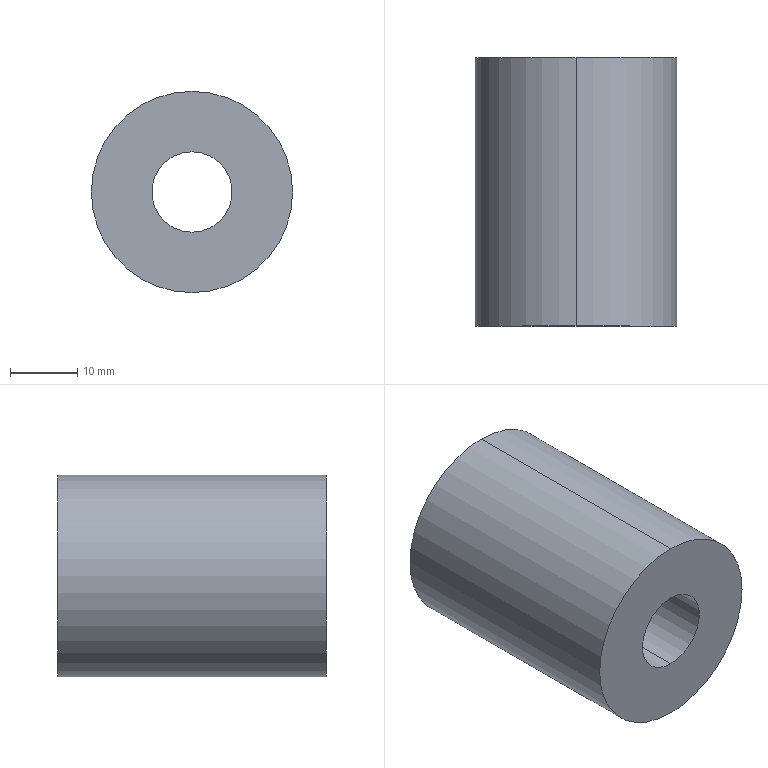Part | SolidWorks | features BaseBody 1 | 1 solid | 6 faces | box 30 x 40 x 30 mm | volume 23750 mm3 | cylinder 4 | plane 2 | commonest cylinder face diameters 12 x2 30 x2
STEP:
#1=CARTESIAN_POINT('',(0.,40.,-15.));
#2=VERTEX_POINT('',#1);
#3=CARTESIAN_POINT('',(0.,40.,15.));
#4=VERTEX_POINT('',#3);
#5=CARTESIAN_POINT('',(0.,40.,0.));
#6=DIRECTION('',(0.,-1.,0.));
#7=DIRECTION('',(0.,0.,-1.));
#8=AXIS2_PLACEMENT_3D('',#5,#6,#7);
#9=CIRCLE('',#8,15.);
#10=EDGE_CURVE('',#2,#4,#9,.T.);
#11=ORIENTED_EDGE('',*,*,#10,.T.);
#12=CARTESIAN_POINT('',(0.,0.,15.));
#13=VERTEX_POINT('',#12);
#14=CARTESIAN_POINT('',(0.,40.,15.));
#15=DIRECTION('',(0.,-1.,0.));
#16=VECTOR('',#15,1000.);
#17=LINE('',#14,#16);
#18=EDGE_CURVE('',#4,#13,#17,.T.);
#19=ORIENTED_EDGE('',*,*,#18,.T.);
#20=CARTESIAN_POINT('',(0.,0.,-15.));
#21=VERTEX_POINT('',#20);
#22=CARTESIAN_POINT('',(0.,0.,0.));
#23=DIRECTION('',(0.,1.,0.));
#24=DIRECTION('',(0.,0.,-1.));
#25=AXIS2_PLACEMENT_3D('',#22,#23,#24);
#26=CIRCLE('',#25,15.);
#27=EDGE_CURVE('',#13,#21,#26,.T.);
#28=ORIENTED_EDGE('',*,*,#27,.T.);
#29=CARTESIAN_POINT('',(0.,40.,-15.));
#30=DIRECTION('',(0.,-1.,0.));
#31=VECTOR('',#30,1000.);
#32=LINE('',#29,#31);
#33=EDGE_CURVE('',#2,#21,#32,.T.);
#34=ORIENTED_EDGE('',*,*,#33,.F.);
#35=EDGE_LOOP('',(#11,#19,#28,#34));
#36=FACE_OUTER_BOUND('',#35,.T.);
#37=CARTESIAN_POINT('',(0.,40.,0.));
#38=DIRECTION('',(0.,-1.,0.));
#39=DIRECTION('',(0.,0.,-1.));
#40=AXIS2_PLACEMENT_3D('',#37,#38,#39);
#41=CYLINDRICAL_SURFACE('',#40,15.);
#42=ADVANCED_FACE('',(#36),#41,.T.);
#43=CARTESIAN_POINT('',(0.,40.,6.));
#44=VERTEX_POINT('',#43);
#45=CARTESIAN_POINT('',(0.,40.,-6.));
#46=VERTEX_POINT('',#45);
#47=CARTESIAN_POINT('',(0.,40.,0.));
#48=DIRECTION('',(0.,-1.,0.));
#49=DIRECTION('',(0.,0.,-1.));
#50=AXIS2_PLACEMENT_3D('',#47,#48,#49);
#51=CIRCLE('',#50,6.);
#52=EDGE_CURVE('',#44,#46,#51,.T.);
#53=ORIENTED_EDGE('',*,*,#52,.F.);
#54=CARTESIAN_POINT('',(0.,0.,6.));
#55=VERTEX_POINT('',#54);
#56=CARTESIAN_POINT('',(0.,40.,6.));
#57=DIRECTION('',(0.,-1.,0.));
#58=VECTOR('',#57,1000.);
#59=LINE('',#56,#58);
#60=EDGE_CURVE('',#44,#55,#59,.T.);
#61=ORIENTED_EDGE('',*,*,#60,.T.);
#62=CARTESIAN_POINT('',(0.,0.,-6.));
#63=VERTEX_POINT('',#62);
#64=CARTESIAN_POINT('',(0.,0.,0.));
#65=DIRECTION('',(0.,-1.,0.));
#66=DIRECTION('',(0.,0.,-1.));
#67=AXIS2_PLACEMENT_3D('',#64,#65,#66);
#68=CIRCLE('',#67,6.);
#69=EDGE_CURVE('',#55,#63,#68,.T.);
#70=ORIENTED_EDGE('',*,*,#69,.T.);
#71=CARTESIAN_POINT('',(0.,40.,-6.));
#72=DIRECTION('',(0.,-1.,0.));
#73=VECTOR('',#72,1000.);
#74=LINE('',#71,#73);
#75=EDGE_CURVE('',#46,#63,#74,.T.);
#76=ORIENTED_EDGE('',*,*,#75,.F.);
#77=EDGE_LOOP('',(#53,#61,#70,#76));
#78=FACE_OUTER_BOUND('',#77,.T.);
#79=CARTESIAN_POINT('',(0.,40.,0.));
#80=DIRECTION('',(0.,-1.,0.));
#81=DIRECTION('',(0.,0.,-1.));
#82=AXIS2_PLACEMENT_3D('',#79,#80,#81);
#83=CYLINDRICAL_SURFACE('',#82,6.);
#84=ADVANCED_FACE('',(#78),#83,.F.);
#85=ORIENTED_EDGE('',*,*,#18,.F.);
#86=CARTESIAN_POINT('',(0.,40.,0.));
#87=DIRECTION('',(0.,-1.,0.));
#88=DIRECTION('',(0.,0.,-1.));
#89=AXIS2_PLACEMENT_3D('',#86,#87,#88);
#90=CIRCLE('',#89,15.);
#91=EDGE_CURVE('',#4,#2,#90,.T.);
#92=ORIENTED_EDGE('',*,*,#91,.T.);
#93=ORIENTED_EDGE('',*,*,#33,.T.);
#94=CARTESIAN_POINT('',(0.,0.,0.));
#95=DIRECTION('',(0.,1.,0.));
#96=DIRECTION('',(0.,0.,-1.));
#97=AXIS2_PLACEMENT_3D('',#94,#95,#96);
#98=CIRCLE('',#97,15.);
#99=EDGE_CURVE('',#21,#13,#98,.T.);
#100=ORIENTED_EDGE('',*,*,#99,.T.);
#101=EDGE_LOOP('',(#85,#92,#93,#100));
#102=FACE_OUTER_BOUND('',#101,.T.);
#103=CARTESIAN_POINT('',(0.,40.,0.));
#104=DIRECTION('',(0.,-1.,0.));
#105=DIRECTION('',(0.,0.,-1.));
#106=AXIS2_PLACEMENT_3D('',#103,#104,#105);
#107=CYLINDRICAL_SURFACE('',#106,15.);
#108=ADVANCED_FACE('',(#102),#107,.T.);
#109=CARTESIAN_POINT('',(0.,0.,0.));
#110=DIRECTION('',(0.,-1.,0.));
#111=DIRECTION('',(0.,0.,-1.));
#112=AXIS2_PLACEMENT_3D('',#109,#110,#111);
#113=CIRCLE('',#112,6.);
#114=EDGE_CURVE('',#63,#55,#113,.T.);
#115=ORIENTED_EDGE('',*,*,#114,.F.);
#116=ORIENTED_EDGE('',*,*,#69,.F.);
#117=EDGE_LOOP('',(#115,#116));
#118=FACE_BOUND('',#117,.T.);
#119=ORIENTED_EDGE('',*,*,#99,.F.);
#120=ORIENTED_EDGE('',*,*,#27,.F.);
#121=EDGE_LOOP('',(#119,#120));
#122=FACE_OUTER_BOUND('',#121,.T.);
#123=CARTESIAN_POINT('',(0.,0.,0.));
#124=DIRECTION('',(0.,1.,0.));
#125=DIRECTION('',(0.,0.,1.));
#126=AXIS2_PLACEMENT_3D('',#123,#124,#125);
#127=PLANE('',#126);
#128=ADVANCED_FACE('',(#118,#122),#127,.F.);
#129=CARTESIAN_POINT('',(0.,40.,0.));
#130=DIRECTION('',(0.,-1.,0.));
#131=DIRECTION('',(0.,0.,-1.));
#132=AXIS2_PLACEMENT_3D('',#129,#130,#131);
#133=CIRCLE('',#132,6.);
#134=EDGE_CURVE('',#46,#44,#133,.T.);
#135=ORIENTED_EDGE('',*,*,#134,.T.);
#136=ORIENTED_EDGE('',*,*,#52,.T.);
#137=EDGE_LOOP('',(#135,#136));
#138=FACE_BOUND('',#137,.T.);
#139=ORIENTED_EDGE('',*,*,#10,.F.);
#140=ORIENTED_EDGE('',*,*,#91,.F.);
#141=EDGE_LOOP('',(#139,#140));
#142=FACE_OUTER_BOUND('',#141,.T.);
#143=CARTESIAN_POINT('',(0.,40.,0.));
#144=DIRECTION('',(0.,1.,0.));
#145=DIRECTION('',(0.,0.,1.));
#146=AXIS2_PLACEMENT_3D('',#143,#144,#145);
#147=PLANE('',#146);
#148=ADVANCED_FACE('',(#138,#142),#147,.T.);
#149=ORIENTED_EDGE('',*,*,#60,.F.);
#150=ORIENTED_EDGE('',*,*,#134,.F.);
#151=ORIENTED_EDGE('',*,*,#75,.T.);
#152=ORIENTED_EDGE('',*,*,#114,.T.);
#153=EDGE_LOOP('',(#149,#150,#151,#152));
#154=FACE_OUTER_BOUND('',#153,.T.);
#155=CARTESIAN_POINT('',(0.,40.,0.));
#156=DIRECTION('',(0.,-1.,0.));
#157=DIRECTION('',(0.,0.,-1.));
#158=AXIS2_PLACEMENT_3D('',#155,#156,#157);
#159=CYLINDRICAL_SURFACE('',#158,6.);
#160=ADVANCED_FACE('',(#154),#159,.F.);
#161=CLOSED_SHELL('',(#42,#84,#108,#128,#148,#160));
#162=MANIFOLD_SOLID_BREP('',#161);
#163=CARTESIAN_POINT('',(0.,0.,0.));
#164=DIRECTION('',(0.,0.,1.));
#165=DIRECTION('',(1.,0.,0.));
#166=AXIS2_PLACEMENT_3D('',#163,#164,#165);
#167=(LENGTH_UNIT()NAMED_UNIT(*)SI_UNIT(.MILLI.,.METRE.));
#168=UNCERTAINTY_MEASURE_WITH_UNIT(LENGTH_MEASURE(0.00001),#167,'','');
#169=(NAMED_UNIT(*)PLANE_ANGLE_UNIT()SI_UNIT($,.RADIAN.));
#170=(NAMED_UNIT(*)SI_UNIT($,.STERADIAN.)SOLID_ANGLE_UNIT());
#171=(GEOMETRIC_REPRESENTATION_CONTEXT(3)GLOBAL_UNCERTAINTY_ASSIGNED_CONTEXT((#168))GLOBAL_UNIT_ASSIGNED_CONTEXT((#167,#169,#170))REPRESENTATION_CONTEXT('',''));
#172=ADVANCED_BREP_SHAPE_REPRESENTATION('',(#162,#166),#171);